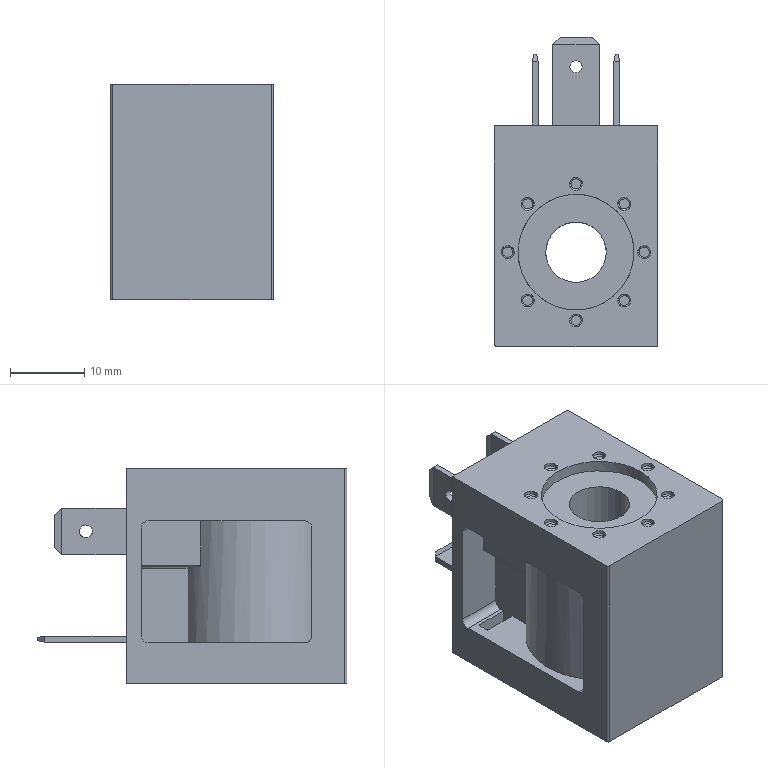Part | SolidWorks | features BaseBody 1 | 1 solid | 177 faces | box 22 x 41.7 x 29 mm | volume 14563 mm3 | plane 73 | cylinder 70 | torus 32 | cone 2 | commonest cylinder face diameters 1.75 x36 0.4 x10 2 x8 15.6 x4 0.6 x2 1.65 x2